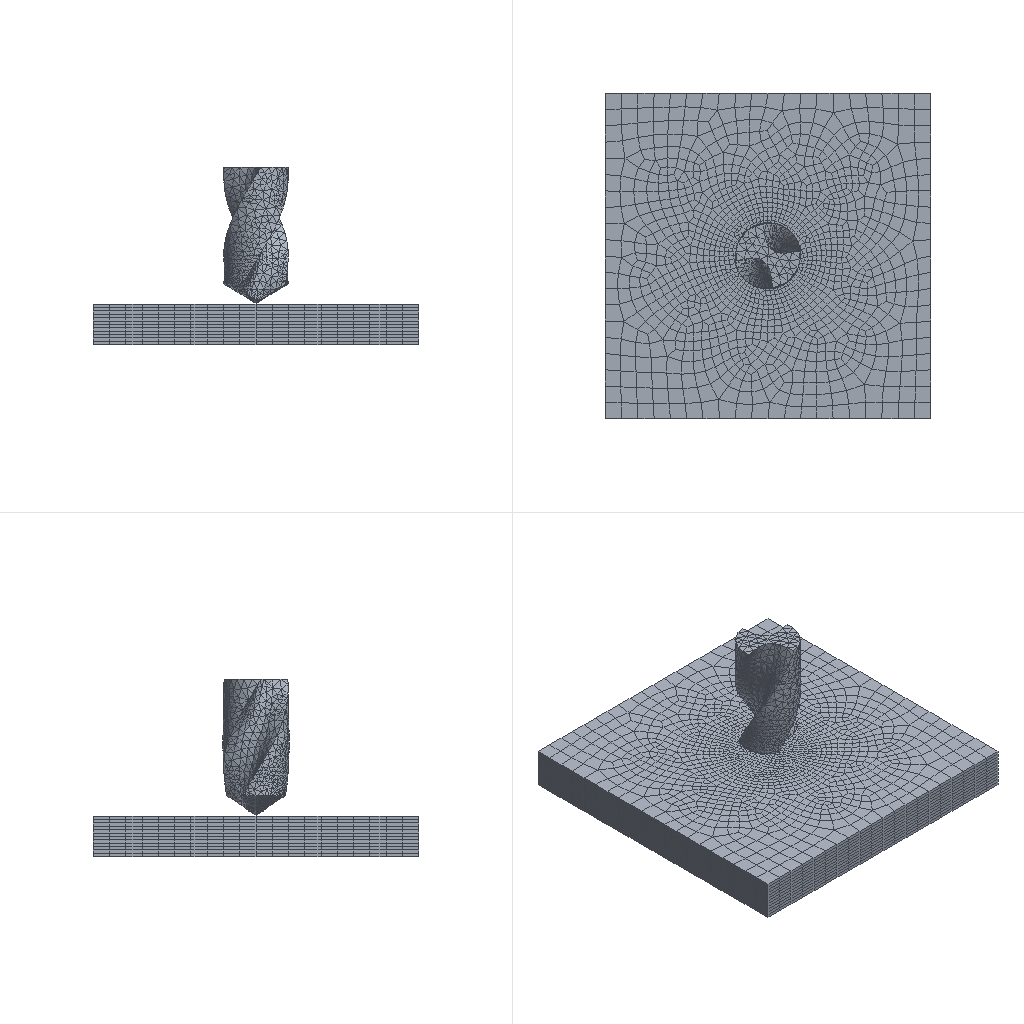Simulation study | abaqus
Set-up summary:
category,name,step,type,value,unit,region
solver,abaqus
solver,version,,,Abaqus/Explicit 3DEXPERIENCE R2017x
units,not stated in the deck,,not stated
analysis,deck,,transient,transient
load_step,Step-1,Step-1,transient
load_step,requested,,,1
mesh,nodes,,,22582
mesh,elements,,,26156
element_type,C3D4,,solid,7388
element_type,C3D8R,,solid,18768
load,load commands in deck,,count,2
bc,support commands in deck,,count,5
material,MATERIAL-1,,in results
material,TOOL,,in results
check,setup vs results,,match,"per instance, exact: element labels, types and connectivity; labels of the nodes the elements use; coordinates not compared"
Abaqus input file, long lists of numbers shortened:
*Heading
** Job name: Job-1 Model name: Model-1
** Generated by: Abaqus/CAE 2017
*Preprint, echo=NO, model=NO, history=NO, contact=NO
**
** PARTS
**
*Part, name=tool
*Node
      1,  -115.53,   1.732,          -1.
      2,  -115.,   1.731,  -1.001
** (1714 more lines like these left out)
*Element, type=C3D4
   1,  885,  886,  887,  888
   2,  886,  889,  890,  891
** (7386 more lines like these left out)
*Node
   1717,  -116.732,           0.,           0.
*Nset, nset=tool-RefPt_, internal
1717,
*Nset, nset=Set-5, generate
    1,  1716,     1
*Elset, elset=Set-5, generate
    1,  7388,     1
** Section: tool
*Solid Section, elset=Set-5, material=tool
,
*End Part
**
*Part, name=work
*Node
      1,           0.,           0.,           0.
      2,          40.,           0.,           0.
** (20863 more lines like these left out)
*Element, type=C3D8R
    1,   146,   145,   335,   339,  2406,  2405,  4797,  4801
    2,   333,   340,   143,   142,  4795,  4802,  2403,  2402
** (18766 more lines like these left out)
*Nset, nset=Set-7, generate
     1,  20865,      1
*Elset, elset=Set-7, generate
     1,  18768,      1
*Orientation, name=Ori-1
1., 0., 0., 0., 1., 0.
1, 0.
** Section: Section-1
*Solid Section, elset=Set-7, orientation=Ori-1, material=Material-1
,
*End Part
**
**
** ASSEMBLY
**
*Assembly, name=Assembly
**
*Instance, name=work-1, part=work
*End Instance
**
*Instance, name=tool-1, part=tool
         20.,         -20.,   121.832
         20.,         -20.,   121.832,          20.,         -21.,   121.832,          90.
*End Instance
**
*Nset, nset=Set-2, instance=work-1
    1,    2,    3,    4,    5,    6,   12,   13,   14,   15,   16,   17,   18,   19,   20,   21
   22,   23,   24,   25,   26,   27,   28,   29,   30,   31,   32,   33,   34,   35,   36,   37
** (72 more lines like these left out)
*Elset, elset=Set-2, instance=work-1, generate
    1,  1106,     1
*Nset, nset=Set-3, instance=tool-1
 1717,
*Nset, nset=Set-4, instance=tool-1
 1717,
*Nset, nset=m_Set-5, instance=tool-1
 1717,
*Nset, nset=s_Set-1, instance=work-1
     5,     6,    11,    88,    89,    90,    91,    92,    93,    94,    95,    96,    97,    98,    99,   100
   101,   102,   103,   104,   105,   106,   107,   108,   109,   110,   111,   112,   113,   114,   115,   116
** (397 more lines like these left out)
*Elset, elset=s_Set-1, instance=work-1, generate
 13273,  18768,      1
*Elset, elset=_m_Surf-1_S4, internal, instance=tool-1
    7,  132,  181,  211,  241,  311,  327,  356,  646,  731, 1082, 1117, 1120, 1122, 1174, 1265
 1309, 1434, 1496, 1536, 1552, 1730, 1795, 1797, 1812, 1836, 1869, 1907, 1913, 1980, 2136, 2198
** (6 more lines like these left out)
*Elset, elset=_m_Surf-1_S3, internal, instance=tool-1
  114,  167,  173,  227,  260,  350,  363,  376,  474,  526,  542,  619,  654,  704,  705,  717
  740,  835,  875,  886,  925,  941,  948,  957, 1064, 1076, 1133, 1215, 1252, 1261, 1277, 1306
** (86 more lines like these left out)
*Elset, elset=_m_Surf-1_S2, internal, instance=tool-1
  243, 1554, 1625, 1643, 1651, 1730, 1797, 1798, 1799, 1865, 1900, 1914, 1966, 1970, 2026, 2135
 2151, 2205, 2221, 2246, 2254, 2298, 2341, 2362, 2363, 2433, 2675, 2700, 2813, 2867, 2928, 2950
** (5 more lines like these left out)
*Elset, elset=_m_Surf-1_S1, internal, instance=tool-1
   69,  168,  221, 1120, 1274, 1310, 1392, 1537, 1578, 1651, 1753, 1878, 1935, 1943, 2226, 2341
 2579, 2674, 2676, 2698, 2857, 3011, 3020, 3025, 3159, 3332, 3353, 3376, 3458, 3558, 3599, 3670
** (3 more lines like these left out)
*Surface, type=ELEMENT, name=m_Surf-1
_m_Surf-1_S4, S4
_m_Surf-1_S3, S3
_m_Surf-1_S2, S2
_m_Surf-1_S1, S1
*Elset, elset=_s_Surf-2_S4, internal, instance=tool-1
   48,  109,  179, 2115, 5517
*Elset, elset=_s_Surf-2_S3, internal, instance=tool-1
  136,  418,  430,  431, 2082, 2264, 2293, 2433, 2441, 2794, 3551, 3552, 4017, 4160, 4181, 4449
 5654, 5655, 6434, 6439, 6445, 6452, 6454, 6462, 6469, 6474, 6477, 6479, 6500, 6503, 6508, 6516
** (1 more lines like these left out)
*Elset, elset=_s_Surf-2_S2, internal, instance=tool-1
  233,  356, 2868, 3025, 3097, 3543, 5675, 6446, 6451
*Elset, elset=_s_Surf-2_S1, internal, instance=tool-1
  241, 2075, 2979, 4171, 5227, 6502
*Surface, type=ELEMENT, name=s_Surf-2
_s_Surf-2_S4, S4
_s_Surf-2_S3, S3
_s_Surf-2_S2, S2
_s_Surf-2_S1, S1
*Surface, type=NODE, name=s_Set-1_CNS_, internal
s_Set-1, 1.
** Constraint: Constraint-1
*Coupling, constraint name=Constraint-1, ref node=m_Set-5, surface=s_Surf-2
*Kinematic
*End Assembly
**
** MATERIALS
**
*Material, name=Material-1
*Density
 1.38e-09,
*Depvar, delete=1
      6,
*Elastic, type=ENGINEERING CONSTANTS
25400.,25400.,71600.,  0.35,  0.25,  0.25, 2100., 2420.
 2420.,
*User Defined Field
*Material, name=tool
*Density
 1.5e-08,
*Elastic
600000., 0.27
**
** INTERACTION PROPERTIES
**
*Surface Interaction, name=IntProp-1
*Friction
 0.2,
*Surface Behavior, pressure-overclosure=HARD
** ----------------------------------------------------------------
**
** STEP: Step-1
**
*Step, name=Step-1, nlgeom=YES
*Dynamic, Explicit
, 0.08
*Bulk Viscosity
0.06, 1.2
** Mass Scaling: Semi-Automatic
**               Whole Model
*Fixed Mass Scaling, factor=1500.
**
** BOUNDARY CONDITIONS
**
** Name: BC-1 Type: 对称/反对称/完全固定
*Boundary
Set-2, ENCASTRE
** Name: BC-2 Type: 速度/角速度
*Boundary, type=VELOCITY
Set-4, 3, 3, -100.
Set-4, 4, 4
Set-4, 5, 5
Set-4, 6, 6, -733.
**
** INTERACTIONS
**
** Interaction: Int-1
*Contact Pair, interaction=IntProp-1, mechanical constraint=KINEMATIC, cpset=Int-1
m_Surf-1, s_Set-1_CNS_
**
** OUTPUT REQUESTS
**
*Restart, write, number interval=1, time marks=NO
**
** FIELD OUTPUT: F-Output-1
**
*Output, field, number interval=100
*Node Output
A, RF, RM, U, V
*Element Output, directions=YES
E, FV, LE, MFR, MISES, PE, PEEQ, PEEQVAVG, PEVAVG, S, SDV, STATUS, SVAVG, UVARM
*Contact Output
CSTRESS,
**
** HISTORY OUTPUT: H-Output-1
**
*Output, history, time interval=8e-05
*Node Output, nset=Set-4
RF1, RF2, RF3, RM1, RM2, RM3, U1, U2
*End Step
Results summary:
result,step,Step-1,completed,increments=306165 time=0.08/0.08
result,analysis,,,transient
result,last_loadstep,,,1
result,primary field,,,U
result,reaction total,,FX,-11563.371,model units
result,reaction total,,FY,6029.736,model units
result,reaction total,,FZ,4171.671,model units